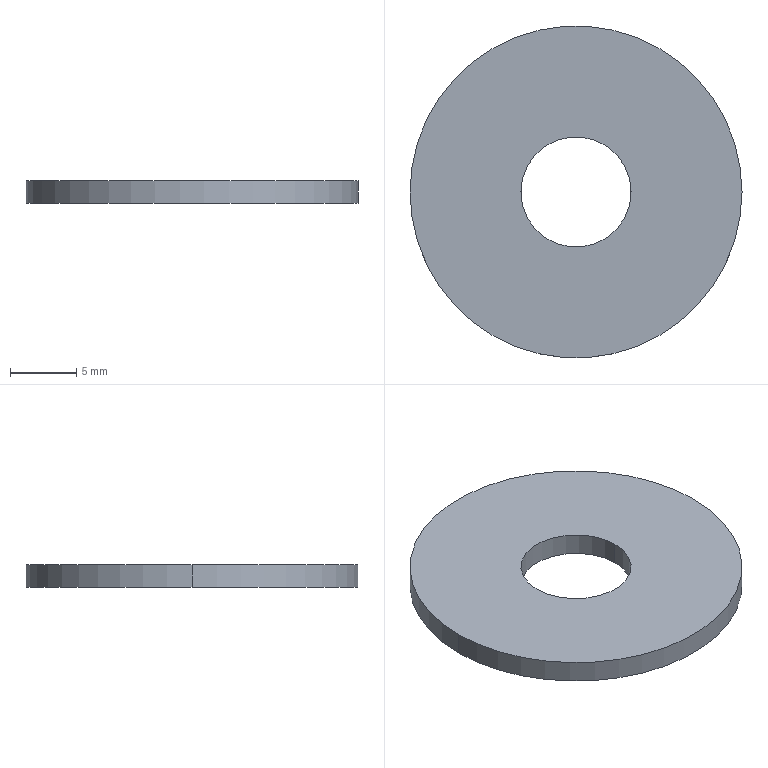Part | SolidWorks | features BaseBody 1 | 1 solid | 6 faces | box 25 x 25 x 1.7 mm | volume 742.505 mm3 | cylinder 4 | plane 2 | commonest cylinder face diameters 8.3 x2 25 x2
STEP:
#1=CARTESIAN_POINT('',(4.15,0.,1.7));
#2=VERTEX_POINT('',#1);
#3=CARTESIAN_POINT('',(-4.15,0.,1.7));
#4=VERTEX_POINT('',#3);
#5=CARTESIAN_POINT('',(0.,0.,1.7));
#6=DIRECTION('',(0.,0.,-1.));
#7=DIRECTION('',(-1.,0.,0.));
#8=AXIS2_PLACEMENT_3D('',#5,#6,#7);
#9=CIRCLE('',#8,4.15);
#10=EDGE_CURVE('',#2,#4,#9,.T.);
#11=ORIENTED_EDGE('',*,*,#10,.F.);
#12=CARTESIAN_POINT('',(4.15,0.,0.));
#13=VERTEX_POINT('',#12);
#14=CARTESIAN_POINT('',(4.15,0.,1.7));
#15=DIRECTION('',(0.,0.,-1.));
#16=VECTOR('',#15,1000.);
#17=LINE('',#14,#16);
#18=EDGE_CURVE('',#2,#13,#17,.T.);
#19=ORIENTED_EDGE('',*,*,#18,.T.);
#20=CARTESIAN_POINT('',(-4.15,0.,0.));
#21=VERTEX_POINT('',#20);
#22=CARTESIAN_POINT('',(0.,0.,0.));
#23=DIRECTION('',(0.,0.,1.));
#24=DIRECTION('',(-1.,0.,0.));
#25=AXIS2_PLACEMENT_3D('',#22,#23,#24);
#26=CIRCLE('',#25,4.15);
#27=EDGE_CURVE('',#21,#13,#26,.T.);
#28=ORIENTED_EDGE('',*,*,#27,.F.);
#29=CARTESIAN_POINT('',(-4.15,0.,1.7));
#30=DIRECTION('',(0.,0.,-1.));
#31=VECTOR('',#30,1000.);
#32=LINE('',#29,#31);
#33=EDGE_CURVE('',#4,#21,#32,.T.);
#34=ORIENTED_EDGE('',*,*,#33,.F.);
#35=EDGE_LOOP('',(#11,#19,#28,#34));
#36=FACE_OUTER_BOUND('',#35,.T.);
#37=CARTESIAN_POINT('',(0.,0.,1.7));
#38=DIRECTION('',(0.,0.,-1.));
#39=DIRECTION('',(-1.,0.,0.));
#40=AXIS2_PLACEMENT_3D('',#37,#38,#39);
#41=CYLINDRICAL_SURFACE('',#40,4.15);
#42=ADVANCED_FACE('',(#36),#41,.F.);
#43=CARTESIAN_POINT('',(12.5,0.,1.7));
#44=VERTEX_POINT('',#43);
#45=CARTESIAN_POINT('',(-12.5,0.,1.7));
#46=VERTEX_POINT('',#45);
#47=CARTESIAN_POINT('',(0.,0.,1.7));
#48=DIRECTION('',(0.,0.,1.));
#49=DIRECTION('',(-1.,0.,0.));
#50=AXIS2_PLACEMENT_3D('',#47,#48,#49);
#51=CIRCLE('',#50,12.5);
#52=EDGE_CURVE('',#44,#46,#51,.T.);
#53=ORIENTED_EDGE('',*,*,#52,.F.);
#54=CARTESIAN_POINT('',(12.5,0.,0.));
#55=VERTEX_POINT('',#54);
#56=CARTESIAN_POINT('',(12.5,0.,1.7));
#57=DIRECTION('',(0.,0.,-1.));
#58=VECTOR('',#57,1000.);
#59=LINE('',#56,#58);
#60=EDGE_CURVE('',#44,#55,#59,.T.);
#61=ORIENTED_EDGE('',*,*,#60,.T.);
#62=CARTESIAN_POINT('',(-12.5,0.,0.));
#63=VERTEX_POINT('',#62);
#64=CARTESIAN_POINT('',(0.,0.,0.));
#65=DIRECTION('',(0.,0.,1.));
#66=DIRECTION('',(-1.,0.,0.));
#67=AXIS2_PLACEMENT_3D('',#64,#65,#66);
#68=CIRCLE('',#67,12.5);
#69=EDGE_CURVE('',#55,#63,#68,.T.);
#70=ORIENTED_EDGE('',*,*,#69,.T.);
#71=CARTESIAN_POINT('',(-12.5,0.,1.7));
#72=DIRECTION('',(0.,0.,-1.));
#73=VECTOR('',#72,1000.);
#74=LINE('',#71,#73);
#75=EDGE_CURVE('',#46,#63,#74,.T.);
#76=ORIENTED_EDGE('',*,*,#75,.F.);
#77=EDGE_LOOP('',(#53,#61,#70,#76));
#78=FACE_OUTER_BOUND('',#77,.T.);
#79=CARTESIAN_POINT('',(0.,0.,1.7));
#80=DIRECTION('',(0.,0.,-1.));
#81=DIRECTION('',(-1.,0.,0.));
#82=AXIS2_PLACEMENT_3D('',#79,#80,#81);
#83=CYLINDRICAL_SURFACE('',#82,12.5);
#84=ADVANCED_FACE('',(#78),#83,.T.);
#85=CARTESIAN_POINT('',(0.,0.,1.7));
#86=DIRECTION('',(0.,0.,-1.));
#87=DIRECTION('',(-1.,0.,0.));
#88=AXIS2_PLACEMENT_3D('',#85,#86,#87);
#89=CIRCLE('',#88,4.15);
#90=EDGE_CURVE('',#4,#2,#89,.T.);
#91=ORIENTED_EDGE('',*,*,#90,.T.);
#92=ORIENTED_EDGE('',*,*,#10,.T.);
#93=EDGE_LOOP('',(#91,#92));
#94=FACE_BOUND('',#93,.T.);
#95=CARTESIAN_POINT('',(0.,0.,1.7));
#96=DIRECTION('',(0.,0.,1.));
#97=DIRECTION('',(-1.,0.,0.));
#98=AXIS2_PLACEMENT_3D('',#95,#96,#97);
#99=CIRCLE('',#98,12.5);
#100=EDGE_CURVE('',#46,#44,#99,.T.);
#101=ORIENTED_EDGE('',*,*,#100,.T.);
#102=ORIENTED_EDGE('',*,*,#52,.T.);
#103=EDGE_LOOP('',(#101,#102));
#104=FACE_OUTER_BOUND('',#103,.T.);
#105=CARTESIAN_POINT('',(0.,0.,1.7));
#106=DIRECTION('',(0.,0.,1.));
#107=DIRECTION('',(1.,0.,0.));
#108=AXIS2_PLACEMENT_3D('',#105,#106,#107);
#109=PLANE('',#108);
#110=ADVANCED_FACE('',(#94,#104),#109,.T.);
#111=ORIENTED_EDGE('',*,*,#18,.F.);
#112=ORIENTED_EDGE('',*,*,#90,.F.);
#113=ORIENTED_EDGE('',*,*,#33,.T.);
#114=CARTESIAN_POINT('',(0.,0.,0.));
#115=DIRECTION('',(0.,0.,1.));
#116=DIRECTION('',(-1.,0.,0.));
#117=AXIS2_PLACEMENT_3D('',#114,#115,#116);
#118=CIRCLE('',#117,4.15);
#119=EDGE_CURVE('',#13,#21,#118,.T.);
#120=ORIENTED_EDGE('',*,*,#119,.F.);
#121=EDGE_LOOP('',(#111,#112,#113,#120));
#122=FACE_OUTER_BOUND('',#121,.T.);
#123=CARTESIAN_POINT('',(0.,0.,1.7));
#124=DIRECTION('',(0.,0.,-1.));
#125=DIRECTION('',(-1.,0.,0.));
#126=AXIS2_PLACEMENT_3D('',#123,#124,#125);
#127=CYLINDRICAL_SURFACE('',#126,4.15);
#128=ADVANCED_FACE('',(#122),#127,.F.);
#129=ORIENTED_EDGE('',*,*,#60,.F.);
#130=ORIENTED_EDGE('',*,*,#100,.F.);
#131=ORIENTED_EDGE('',*,*,#75,.T.);
#132=CARTESIAN_POINT('',(0.,0.,0.));
#133=DIRECTION('',(0.,0.,1.));
#134=DIRECTION('',(-1.,0.,0.));
#135=AXIS2_PLACEMENT_3D('',#132,#133,#134);
#136=CIRCLE('',#135,12.5);
#137=EDGE_CURVE('',#63,#55,#136,.T.);
#138=ORIENTED_EDGE('',*,*,#137,.T.);
#139=EDGE_LOOP('',(#129,#130,#131,#138));
#140=FACE_OUTER_BOUND('',#139,.T.);
#141=CARTESIAN_POINT('',(0.,0.,1.7));
#142=DIRECTION('',(0.,0.,-1.));
#143=DIRECTION('',(-1.,0.,0.));
#144=AXIS2_PLACEMENT_3D('',#141,#142,#143);
#145=CYLINDRICAL_SURFACE('',#144,12.5);
#146=ADVANCED_FACE('',(#140),#145,.T.);
#147=ORIENTED_EDGE('',*,*,#27,.T.);
#148=ORIENTED_EDGE('',*,*,#119,.T.);
#149=EDGE_LOOP('',(#147,#148));
#150=FACE_BOUND('',#149,.T.);
#151=ORIENTED_EDGE('',*,*,#137,.F.);
#152=ORIENTED_EDGE('',*,*,#69,.F.);
#153=EDGE_LOOP('',(#151,#152));
#154=FACE_OUTER_BOUND('',#153,.T.);
#155=CARTESIAN_POINT('',(0.,0.,0.));
#156=DIRECTION('',(0.,0.,1.));
#157=DIRECTION('',(1.,0.,0.));
#158=AXIS2_PLACEMENT_3D('',#155,#156,#157);
#159=PLANE('',#158);
#160=ADVANCED_FACE('',(#150,#154),#159,.F.);
#161=CLOSED_SHELL('',(#42,#84,#110,#128,#146,#160));
#162=MANIFOLD_SOLID_BREP('',#161);
#163=CARTESIAN_POINT('',(0.,0.,0.));
#164=DIRECTION('',(0.,0.,1.));
#165=DIRECTION('',(1.,0.,0.));
#166=AXIS2_PLACEMENT_3D('',#163,#164,#165);
#167=(LENGTH_UNIT()NAMED_UNIT(*)SI_UNIT(.MILLI.,.METRE.));
#168=UNCERTAINTY_MEASURE_WITH_UNIT(LENGTH_MEASURE(0.00001),#167,'','');
#169=(NAMED_UNIT(*)PLANE_ANGLE_UNIT()SI_UNIT($,.RADIAN.));
#170=(NAMED_UNIT(*)SI_UNIT($,.STERADIAN.)SOLID_ANGLE_UNIT());
#171=(GEOMETRIC_REPRESENTATION_CONTEXT(3)GLOBAL_UNCERTAINTY_ASSIGNED_CONTEXT((#168))GLOBAL_UNIT_ASSIGNED_CONTEXT((#167,#169,#170))REPRESENTATION_CONTEXT('',''));
#172=ADVANCED_BREP_SHAPE_REPRESENTATION('',(#162,#166),#171);